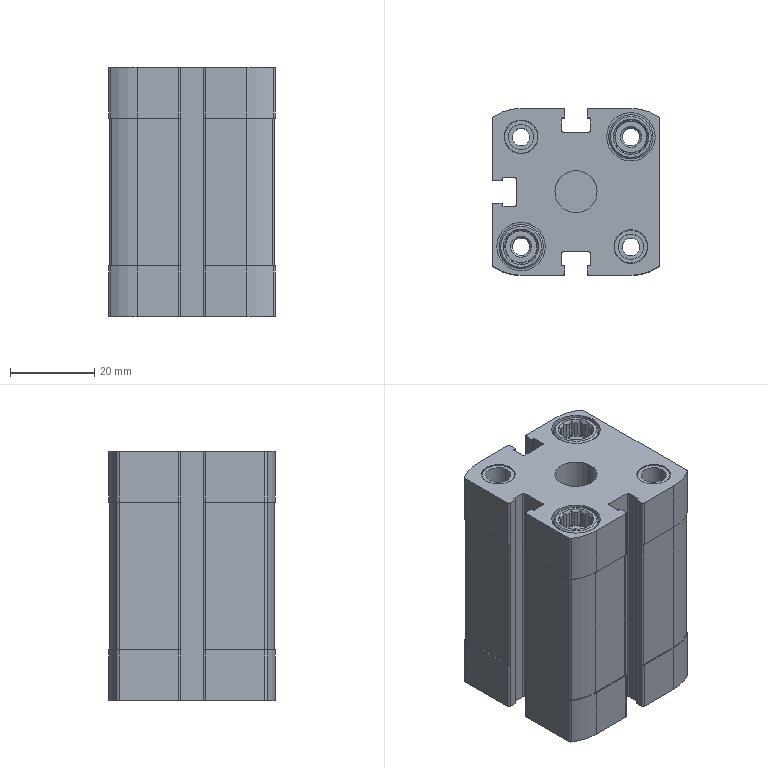Part | NX | features BREP 1 | 1 solid | 330 faces | box 39.5 x 39.5 x 59 mm | volume 61872 mm3 | plane 221 | cylinder 91 | cone 18 | commonest cylinder face diameters 0.8 x24 0.4 x12 1.6 x12 23.4 x12 4.134 x8 6 x4